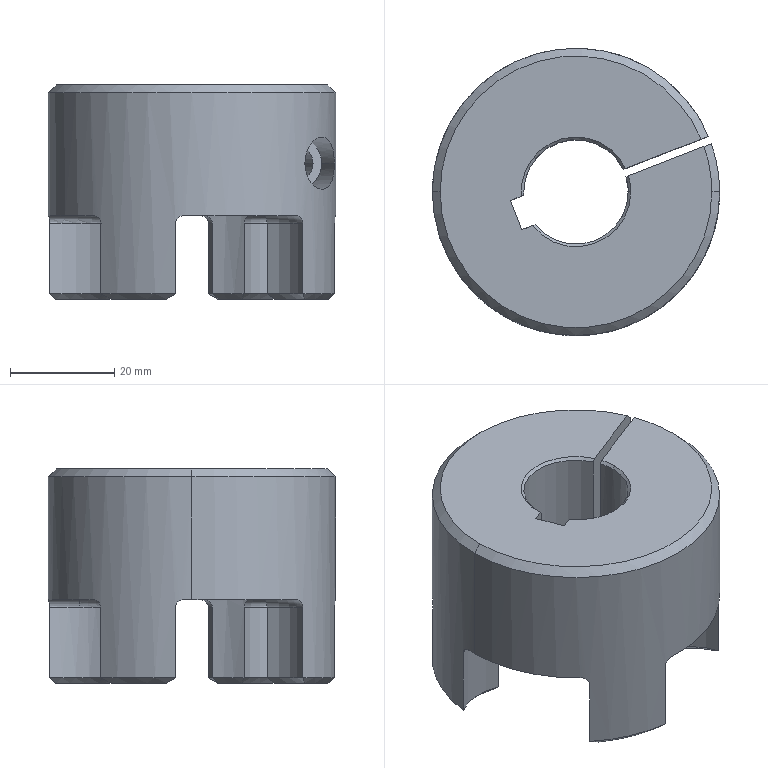Part | NX | features BREP 1 | 1 solid | 76 faces | box 55 x 55 x 41 mm | volume 54768 mm3 | cone 26 | cylinder 24 | plane 17 | torus 9 | commonest cylinder face diameters 22.734 x9 20 x3 35 x3 55 x3 5 x2 6.5 x2